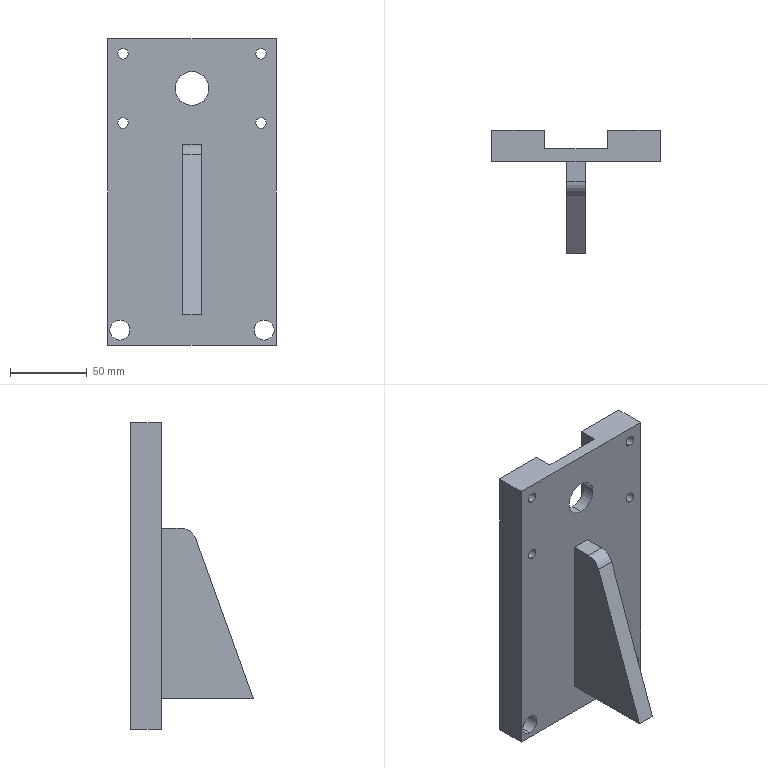Part | SolidWorks | features BaseBody 1 | 1 solid | 30 faces | box 110 x 80 x 200 mm | volume 383509 mm3 | cylinder 15 | plane 15 | commonest cylinder face diameters 6.8 x8 13 x4 22 x2 20 x1
STEP:
#1=CARTESIAN_POINT('',(178.,130.,-29.379));
#2=VERTEX_POINT('',#1);
#3=CARTESIAN_POINT('',(178.,130.,-16.379));
#4=VERTEX_POINT('',#3);
#5=CARTESIAN_POINT('',(178.,130.,-22.879));
#6=DIRECTION('',(0.,1.,0.));
#7=DIRECTION('',(0.,0.,1.));
#8=AXIS2_PLACEMENT_3D('',#5,#6,#7);
#9=CIRCLE('',#8,6.5);
#10=EDGE_CURVE('',#2,#4,#9,.T.);
#11=ORIENTED_EDGE('',*,*,#10,.F.);
#12=CARTESIAN_POINT('',(178.,150.,-29.379));
#13=VERTEX_POINT('',#12);
#14=CARTESIAN_POINT('',(178.,130.,-29.379));
#15=DIRECTION('',(0.,1.,0.));
#16=VECTOR('',#15,1000.);
#17=LINE('',#14,#16);
#18=EDGE_CURVE('',#2,#13,#17,.T.);
#19=ORIENTED_EDGE('',*,*,#18,.T.);
#20=CARTESIAN_POINT('',(178.,150.,-16.379));
#21=VERTEX_POINT('',#20);
#22=CARTESIAN_POINT('',(178.,150.,-22.879));
#23=DIRECTION('',(0.,-1.,0.));
#24=DIRECTION('',(0.,0.,1.));
#25=AXIS2_PLACEMENT_3D('',#22,#23,#24);
#26=CIRCLE('',#25,6.5);
#27=EDGE_CURVE('',#21,#13,#26,.T.);
#28=ORIENTED_EDGE('',*,*,#27,.F.);
#29=CARTESIAN_POINT('',(178.,130.,-16.379));
#30=DIRECTION('',(0.,1.,0.));
#31=VECTOR('',#30,1000.);
#32=LINE('',#29,#31);
#33=EDGE_CURVE('',#4,#21,#32,.T.);
#34=ORIENTED_EDGE('',*,*,#33,.F.);
#35=EDGE_LOOP('',(#11,#19,#28,#34));
#36=FACE_OUTER_BOUND('',#35,.T.);
#37=CARTESIAN_POINT('',(178.,130.,-22.879));
#38=DIRECTION('',(0.,1.,0.));
#39=DIRECTION('',(0.,0.,1.));
#40=AXIS2_PLACEMENT_3D('',#37,#38,#39);
#41=CYLINDRICAL_SURFACE('',#40,6.5);
#42=ADVANCED_FACE('',(#36),#41,.F.);
#43=CARTESIAN_POINT('',(272.,130.,-29.379));
#44=VERTEX_POINT('',#43);
#45=CARTESIAN_POINT('',(272.,130.,-16.379));
#46=VERTEX_POINT('',#45);
#47=CARTESIAN_POINT('',(272.,130.,-22.879));
#48=DIRECTION('',(0.,1.,0.));
#49=DIRECTION('',(0.,0.,1.));
#50=AXIS2_PLACEMENT_3D('',#47,#48,#49);
#51=CIRCLE('',#50,6.5);
#52=EDGE_CURVE('',#44,#46,#51,.T.);
#53=ORIENTED_EDGE('',*,*,#52,.F.);
#54=CARTESIAN_POINT('',(272.,150.,-29.379));
#55=VERTEX_POINT('',#54);
#56=CARTESIAN_POINT('',(272.,130.,-29.379));
#57=DIRECTION('',(0.,1.,0.));
#58=VECTOR('',#57,1000.);
#59=LINE('',#56,#58);
#60=EDGE_CURVE('',#44,#55,#59,.T.);
#61=ORIENTED_EDGE('',*,*,#60,.T.);
#62=CARTESIAN_POINT('',(272.,150.,-16.379));
#63=VERTEX_POINT('',#62);
#64=CARTESIAN_POINT('',(272.,150.,-22.879));
#65=DIRECTION('',(0.,-1.,0.));
#66=DIRECTION('',(0.,0.,1.));
#67=AXIS2_PLACEMENT_3D('',#64,#65,#66);
#68=CIRCLE('',#67,6.5);
#69=EDGE_CURVE('',#63,#55,#68,.T.);
#70=ORIENTED_EDGE('',*,*,#69,.F.);
#71=CARTESIAN_POINT('',(272.,130.,-16.379));
#72=DIRECTION('',(0.,1.,0.));
#73=VECTOR('',#72,1000.);
#74=LINE('',#71,#73);
#75=EDGE_CURVE('',#46,#63,#74,.T.);
#76=ORIENTED_EDGE('',*,*,#75,.F.);
#77=EDGE_LOOP('',(#53,#61,#70,#76));
#78=FACE_OUTER_BOUND('',#77,.T.);
#79=CARTESIAN_POINT('',(272.,130.,-22.879));
#80=DIRECTION('',(0.,1.,0.));
#81=DIRECTION('',(0.,0.,1.));
#82=AXIS2_PLACEMENT_3D('',#79,#80,#81);
#83=CYLINDRICAL_SURFACE('',#82,6.5);
#84=ADVANCED_FACE('',(#78),#83,.F.);
#85=CARTESIAN_POINT('',(270.,130.,108.721));
#86=VERTEX_POINT('',#85);
#87=CARTESIAN_POINT('',(270.,130.,115.521));
#88=VERTEX_POINT('',#87);
#89=CARTESIAN_POINT('',(270.,130.,112.121));
#90=DIRECTION('',(0.,1.,0.));
#91=DIRECTION('',(0.,0.,1.));
#92=AXIS2_PLACEMENT_3D('',#89,#90,#91);
#93=CIRCLE('',#92,3.4);
#94=EDGE_CURVE('',#86,#88,#93,.T.);
#95=ORIENTED_EDGE('',*,*,#94,.F.);
#96=CARTESIAN_POINT('',(270.,150.,108.721));
#97=VERTEX_POINT('',#96);
#98=CARTESIAN_POINT('',(270.,150.,108.721));
#99=DIRECTION('',(0.,1.,0.));
#100=VECTOR('',#99,1000.);
#101=LINE('',#98,#100);
#102=EDGE_CURVE('',#86,#97,#101,.T.);
#103=ORIENTED_EDGE('',*,*,#102,.T.);
#104=CARTESIAN_POINT('',(270.,150.,115.521));
#105=VERTEX_POINT('',#104);
#106=CARTESIAN_POINT('',(270.,150.,112.121));
#107=DIRECTION('',(0.,-1.,0.));
#108=DIRECTION('',(0.,0.,1.));
#109=AXIS2_PLACEMENT_3D('',#106,#107,#108);
#110=CIRCLE('',#109,3.4);
#111=EDGE_CURVE('',#105,#97,#110,.T.);
#112=ORIENTED_EDGE('',*,*,#111,.F.);
#113=CARTESIAN_POINT('',(270.,150.,115.521));
#114=DIRECTION('',(0.,1.,0.));
#115=VECTOR('',#114,1000.);
#116=LINE('',#113,#115);
#117=EDGE_CURVE('',#88,#105,#116,.T.);
#118=ORIENTED_EDGE('',*,*,#117,.F.);
#119=EDGE_LOOP('',(#95,#103,#112,#118));
#120=FACE_OUTER_BOUND('',#119,.T.);
#121=CARTESIAN_POINT('',(270.,150.,112.121));
#122=DIRECTION('',(0.,1.,0.));
#123=DIRECTION('',(0.,0.,1.));
#124=AXIS2_PLACEMENT_3D('',#121,#122,#123);
#125=CYLINDRICAL_SURFACE('',#124,3.4);
#126=ADVANCED_FACE('',(#120),#125,.F.);
#127=CARTESIAN_POINT('',(270.,130.,153.721));
#128=VERTEX_POINT('',#127);
#129=CARTESIAN_POINT('',(270.,130.,160.521));
#130=VERTEX_POINT('',#129);
#131=CARTESIAN_POINT('',(270.,130.,157.121));
#132=DIRECTION('',(0.,1.,0.));
#133=DIRECTION('',(0.,0.,1.));
#134=AXIS2_PLACEMENT_3D('',#131,#132,#133);
#135=CIRCLE('',#134,3.4);
#136=EDGE_CURVE('',#128,#130,#135,.T.);
#137=ORIENTED_EDGE('',*,*,#136,.F.);
#138=CARTESIAN_POINT('',(270.,150.,153.721));
#139=VERTEX_POINT('',#138);
#140=CARTESIAN_POINT('',(270.,150.,153.721));
#141=DIRECTION('',(0.,1.,0.));
#142=VECTOR('',#141,1000.);
#143=LINE('',#140,#142);
#144=EDGE_CURVE('',#128,#139,#143,.T.);
#145=ORIENTED_EDGE('',*,*,#144,.T.);
#146=CARTESIAN_POINT('',(270.,150.,160.521));
#147=VERTEX_POINT('',#146);
#148=CARTESIAN_POINT('',(270.,150.,157.121));
#149=DIRECTION('',(0.,-1.,0.));
#150=DIRECTION('',(0.,0.,1.));
#151=AXIS2_PLACEMENT_3D('',#148,#149,#150);
#152=CIRCLE('',#151,3.4);
#153=EDGE_CURVE('',#147,#139,#152,.T.);
#154=ORIENTED_EDGE('',*,*,#153,.F.);
#155=CARTESIAN_POINT('',(270.,150.,160.521));
#156=DIRECTION('',(0.,1.,0.));
#157=VECTOR('',#156,1000.);
#158=LINE('',#155,#157);
#159=EDGE_CURVE('',#130,#147,#158,.T.);
#160=ORIENTED_EDGE('',*,*,#159,.F.);
#161=EDGE_LOOP('',(#137,#145,#154,#160));
#162=FACE_OUTER_BOUND('',#161,.T.);
#163=CARTESIAN_POINT('',(270.,150.,157.121));
#164=DIRECTION('',(0.,1.,0.));
#165=DIRECTION('',(0.,0.,1.));
#166=AXIS2_PLACEMENT_3D('',#163,#164,#165);
#167=CYLINDRICAL_SURFACE('',#166,3.4);
#168=ADVANCED_FACE('',(#162),#167,.F.);
#169=CARTESIAN_POINT('',(180.,130.,108.721));
#170=VERTEX_POINT('',#169);
#171=CARTESIAN_POINT('',(180.,130.,115.521));
#172=VERTEX_POINT('',#171);
#173=CARTESIAN_POINT('',(180.,130.,112.121));
#174=DIRECTION('',(0.,1.,0.));
#175=DIRECTION('',(0.,0.,1.));
#176=AXIS2_PLACEMENT_3D('',#173,#174,#175);
#177=CIRCLE('',#176,3.4);
#178=EDGE_CURVE('',#170,#172,#177,.T.);
#179=ORIENTED_EDGE('',*,*,#178,.F.);
#180=CARTESIAN_POINT('',(180.,150.,108.721));
#181=VERTEX_POINT('',#180);
#182=CARTESIAN_POINT('',(180.,150.,108.721));
#183=DIRECTION('',(0.,1.,0.));
#184=VECTOR('',#183,1000.);
#185=LINE('',#182,#184);
#186=EDGE_CURVE('',#170,#181,#185,.T.);
#187=ORIENTED_EDGE('',*,*,#186,.T.);
#188=CARTESIAN_POINT('',(180.,150.,115.521));
#189=VERTEX_POINT('',#188);
#190=CARTESIAN_POINT('',(180.,150.,112.121));
#191=DIRECTION('',(0.,-1.,0.));
#192=DIRECTION('',(0.,0.,1.));
#193=AXIS2_PLACEMENT_3D('',#190,#191,#192);
#194=CIRCLE('',#193,3.4);
#195=EDGE_CURVE('',#189,#181,#194,.T.);
#196=ORIENTED_EDGE('',*,*,#195,.F.);
#197=CARTESIAN_POINT('',(180.,150.,115.521));
#198=DIRECTION('',(0.,1.,0.));
#199=VECTOR('',#198,1000.);
#200=LINE('',#197,#199);
#201=EDGE_CURVE('',#172,#189,#200,.T.);
#202=ORIENTED_EDGE('',*,*,#201,.F.);
#203=EDGE_LOOP('',(#179,#187,#196,#202));
#204=FACE_OUTER_BOUND('',#203,.T.);
#205=CARTESIAN_POINT('',(180.,150.,112.121));
#206=DIRECTION('',(0.,1.,0.));
#207=DIRECTION('',(0.,0.,1.));
#208=AXIS2_PLACEMENT_3D('',#205,#206,#207);
#209=CYLINDRICAL_SURFACE('',#208,3.4);
#210=ADVANCED_FACE('',(#204),#209,.F.);
#211=CARTESIAN_POINT('',(180.,130.,153.721));
#212=VERTEX_POINT('',#211);
#213=CARTESIAN_POINT('',(180.,130.,160.521));
#214=VERTEX_POINT('',#213);
#215=CARTESIAN_POINT('',(180.,130.,157.121));
#216=DIRECTION('',(0.,1.,0.));
#217=DIRECTION('',(0.,0.,1.));
#218=AXIS2_PLACEMENT_3D('',#215,#216,#217);
#219=CIRCLE('',#218,3.4);
#220=EDGE_CURVE('',#212,#214,#219,.T.);
#221=ORIENTED_EDGE('',*,*,#220,.F.);
#222=CARTESIAN_POINT('',(180.,150.,153.721));
#223=VERTEX_POINT('',#222);
#224=CARTESIAN_POINT('',(180.,150.,153.721));
#225=DIRECTION('',(0.,1.,0.));
#226=VECTOR('',#225,1000.);
#227=LINE('',#224,#226);
#228=EDGE_CURVE('',#212,#223,#227,.T.);
#229=ORIENTED_EDGE('',*,*,#228,.T.);
#230=CARTESIAN_POINT('',(180.,150.,160.521));
#231=VERTEX_POINT('',#230);
#232=CARTESIAN_POINT('',(180.,150.,157.121));
#233=DIRECTION('',(0.,-1.,0.));
#234=DIRECTION('',(0.,0.,1.));
#235=AXIS2_PLACEMENT_3D('',#232,#233,#234);
#236=CIRCLE('',#235,3.4);
#237=EDGE_CURVE('',#231,#223,#236,.T.);
#238=ORIENTED_EDGE('',*,*,#237,.F.);
#239=CARTESIAN_POINT('',(180.,150.,160.521));
#240=DIRECTION('',(0.,1.,0.));
#241=VECTOR('',#240,1000.);
#242=LINE('',#239,#241);
#243=EDGE_CURVE('',#214,#231,#242,.T.);
#244=ORIENTED_EDGE('',*,*,#243,.F.);
#245=EDGE_LOOP('',(#221,#229,#238,#244));
#246=FACE_OUTER_BOUND('',#245,.T.);
#247=CARTESIAN_POINT('',(180.,150.,157.121));
#248=DIRECTION('',(0.,1.,0.));
#249=DIRECTION('',(0.,0.,1.));
#250=AXIS2_PLACEMENT_3D('',#247,#248,#249);
#251=CYLINDRICAL_SURFACE('',#250,3.4);
#252=ADVANCED_FACE('',(#246),#251,.F.);
#253=CARTESIAN_POINT('',(225.,130.,123.621));
#254=VERTEX_POINT('',#253);
#255=CARTESIAN_POINT('',(225.,130.,145.621));
#256=VERTEX_POINT('',#255);
#257=CARTESIAN_POINT('',(225.,130.,134.621));
#258=DIRECTION('',(0.,1.,0.));
#259=DIRECTION('',(0.,0.,1.));
#260=AXIS2_PLACEMENT_3D('',#257,#258,#259);
#261=CIRCLE('',#260,11.);
#262=EDGE_CURVE('',#254,#256,#261,.T.);
#263=ORIENTED_EDGE('',*,*,#262,.F.);
#264=CARTESIAN_POINT('',(225.,138.,123.621));
#265=VERTEX_POINT('',#264);
#266=CARTESIAN_POINT('',(225.,129.999,123.621));
#267=DIRECTION('',(0.,1.,0.));
#268=VECTOR('',#267,1000.);
#269=LINE('',#266,#268);
#270=EDGE_CURVE('',#254,#265,#269,.T.);
#271=ORIENTED_EDGE('',*,*,#270,.T.);
#272=CARTESIAN_POINT('',(225.,138.,145.621));
#273=VERTEX_POINT('',#272);
#274=CARTESIAN_POINT('',(225.,138.,134.621));
#275=DIRECTION('',(0.,-1.,0.));
#276=DIRECTION('',(0.,0.,1.));
#277=AXIS2_PLACEMENT_3D('',#274,#275,#276);
#278=CIRCLE('',#277,11.);
#279=EDGE_CURVE('',#273,#265,#278,.T.);
#280=ORIENTED_EDGE('',*,*,#279,.F.);
#281=CARTESIAN_POINT('',(225.,129.999,145.621));
#282=DIRECTION('',(0.,1.,0.));
#283=VECTOR('',#282,1000.);
#284=LINE('',#281,#283);
#285=EDGE_CURVE('',#256,#273,#284,.T.);
#286=ORIENTED_EDGE('',*,*,#285,.F.);
#287=EDGE_LOOP('',(#263,#271,#280,#286));
#288=FACE_OUTER_BOUND('',#287,.T.);
#289=CARTESIAN_POINT('',(225.,129.999,134.621));
#290=DIRECTION('',(0.,1.,0.));
#291=DIRECTION('',(0.,0.,1.));
#292=AXIS2_PLACEMENT_3D('',#289,#290,#291);
#293=CYLINDRICAL_SURFACE('',#292,11.);
#294=ADVANCED_FACE('',(#288),#293,.F.);
#295=CARTESIAN_POINT('',(231.,130.,-12.879));
#296=VERTEX_POINT('',#295);
#297=CARTESIAN_POINT('',(219.,130.,-12.879));
#298=VERTEX_POINT('',#297);
#299=CARTESIAN_POINT('',(225.,130.,-12.879));
#300=DIRECTION('',(-1.,0.,0.));
#301=VECTOR('',#300,1000.);
#302=LINE('',#299,#301);
#303=EDGE_CURVE('',#296,#298,#302,.T.);
#304=ORIENTED_EDGE('',*,*,#303,.T.);
#305=CARTESIAN_POINT('',(219.,130.,98.107));
#306=VERTEX_POINT('',#305);
#307=CARTESIAN_POINT('',(219.,130.,67.121));
#308=DIRECTION('',(0.,0.,1.));
#309=VECTOR('',#308,1000.);
#310=LINE('',#307,#309);
#311=EDGE_CURVE('',#298,#306,#310,.T.);
#312=ORIENTED_EDGE('',*,*,#311,.T.);
#313=CARTESIAN_POINT('',(231.,130.,98.107));
#314=VERTEX_POINT('',#313);
#315=CARTESIAN_POINT('',(225.,130.,98.107));
#316=DIRECTION('',(1.,0.,0.));
#317=VECTOR('',#316,1000.);
#318=LINE('',#315,#317);
#319=EDGE_CURVE('',#306,#314,#318,.T.);
#320=ORIENTED_EDGE('',*,*,#319,.T.);
#321=CARTESIAN_POINT('',(231.,130.,67.121));
#322=DIRECTION('',(0.,0.,-1.));
#323=VECTOR('',#322,1000.);
#324=LINE('',#321,#323);
#325=EDGE_CURVE('',#314,#296,#324,.T.);
#326=ORIENTED_EDGE('',*,*,#325,.T.);
#327=EDGE_LOOP('',(#304,#312,#320,#326));
#328=FACE_BOUND('',#327,.T.);
#329=CARTESIAN_POINT('',(178.,130.,-22.879));
#330=DIRECTION('',(0.,1.,0.));
#331=DIRECTION('',(0.,0.,1.));
#332=AXIS2_PLACEMENT_3D('',#329,#330,#331);
#333=CIRCLE('',#332,6.5);
#334=EDGE_CURVE('',#4,#2,#333,.T.);
#335=ORIENTED_EDGE('',*,*,#334,.T.);
#336=ORIENTED_EDGE('',*,*,#10,.T.);
#337=EDGE_LOOP('',(#335,#336));
#338=FACE_BOUND('',#337,.T.);
#339=CARTESIAN_POINT('',(272.,130.,-22.879));
#340=DIRECTION('',(0.,1.,0.));
#341=DIRECTION('',(0.,0.,1.));
#342=AXIS2_PLACEMENT_3D('',#339,#340,#341);
#343=CIRCLE('',#342,6.5);
#344=EDGE_CURVE('',#46,#44,#343,.T.);
#345=ORIENTED_EDGE('',*,*,#344,.T.);
#346=ORIENTED_EDGE('',*,*,#52,.T.);
#347=EDGE_LOOP('',(#345,#346));
#348=FACE_BOUND('',#347,.T.);
#349=CARTESIAN_POINT('',(270.,130.,112.121));
#350=DIRECTION('',(0.,1.,0.));
#351=DIRECTION('',(0.,0.,1.));
#352=AXIS2_PLACEMENT_3D('',#349,#350,#351);
#353=CIRCLE('',#352,3.4);
#354=EDGE_CURVE('',#88,#86,#353,.T.);
#355=ORIENTED_EDGE('',*,*,#354,.T.);
#356=ORIENTED_EDGE('',*,*,#94,.T.);
#357=EDGE_LOOP('',(#355,#356));
#358=FACE_BOUND('',#357,.T.);
#359=CARTESIAN_POINT('',(270.,130.,157.121));
#360=DIRECTION('',(0.,1.,0.));
#361=DIRECTION('',(0.,0.,1.));
#362=AXIS2_PLACEMENT_3D('',#359,#360,#361);
#363=CIRCLE('',#362,3.4);
#364=EDGE_CURVE('',#130,#128,#363,.T.);
#365=ORIENTED_EDGE('',*,*,#364,.T.);
#366=ORIENTED_EDGE('',*,*,#136,.T.);
#367=EDGE_LOOP('',(#365,#366));
#368=FACE_BOUND('',#367,.T.);
#369=CARTESIAN_POINT('',(180.,130.,112.121));
#370=DIRECTION('',(0.,1.,0.));
#371=DIRECTION('',(0.,0.,1.));
#372=AXIS2_PLACEMENT_3D('',#369,#370,#371);
#373=CIRCLE('',#372,3.4);
#374=EDGE_CURVE('',#172,#170,#373,.T.);
#375=ORIENTED_EDGE('',*,*,#374,.T.);
#376=ORIENTED_EDGE('',*,*,#178,.T.);
#377=EDGE_LOOP('',(#375,#376));
#378=FACE_BOUND('',#377,.T.);
#379=CARTESIAN_POINT('',(180.,130.,157.121));
#380=DIRECTION('',(0.,1.,0.));
#381=DIRECTION('',(0.,0.,1.));
#382=AXIS2_PLACEMENT_3D('',#379,#380,#381);
#383=CIRCLE('',#382,3.4);
#384=EDGE_CURVE('',#214,#212,#383,.T.);
#385=ORIENTED_EDGE('',*,*,#384,.T.);
#386=ORIENTED_EDGE('',*,*,#220,.T.);
#387=EDGE_LOOP('',(#385,#386));
#388=FACE_BOUND('',#387,.T.);
#389=CARTESIAN_POINT('',(225.,130.,134.621));
#390=DIRECTION('',(0.,1.,0.));
#391=DIRECTION('',(0.,0.,1.));
#392=AXIS2_PLACEMENT_3D('',#389,#390,#391);
#393=CIRCLE('',#392,11.);
#394=EDGE_CURVE('',#256,#254,#393,.T.);
#395=ORIENTED_EDGE('',*,*,#394,.T.);
#396=ORIENTED_EDGE('',*,*,#262,.T.);
#397=EDGE_LOOP('',(#395,#396));
#398=FACE_BOUND('',#397,.T.);
#399=CARTESIAN_POINT('',(170.,130.,167.121));
#400=VERTEX_POINT('',#399);
#401=CARTESIAN_POINT('',(170.,130.,-32.879));
#402=VERTEX_POINT('',#401);
#403=CARTESIAN_POINT('',(170.,130.,67.121));
#404=DIRECTION('',(0.,0.,-1.));
#405=VECTOR('',#404,1000.);
#406=LINE('',#403,#405);
#407=EDGE_CURVE('',#400,#402,#406,.T.);
#408=ORIENTED_EDGE('',*,*,#407,.T.);
#409=CARTESIAN_POINT('',(280.,130.,-32.879));
#410=VERTEX_POINT('',#409);
#411=CARTESIAN_POINT('',(225.,130.,-32.879));
#412=DIRECTION('',(1.,0.,0.));
#413=VECTOR('',#412,1000.);
#414=LINE('',#411,#413);
#415=EDGE_CURVE('',#402,#410,#414,.T.);
#416=ORIENTED_EDGE('',*,*,#415,.T.);
#417=CARTESIAN_POINT('',(280.,130.,167.121));
#418=VERTEX_POINT('',#417);
#419=CARTESIAN_POINT('',(280.,130.,67.121));
#420=DIRECTION('',(0.,0.,1.));
#421=VECTOR('',#420,1000.);
#422=LINE('',#419,#421);
#423=EDGE_CURVE('',#410,#418,#422,.T.);
#424=ORIENTED_EDGE('',*,*,#423,.T.);
#425=CARTESIAN_POINT('',(225.,130.,167.121));
#426=DIRECTION('',(-1.,0.,0.));
#427=VECTOR('',#426,1000.);
#428=LINE('',#425,#427);
#429=EDGE_CURVE('',#418,#400,#428,.T.);
#430=ORIENTED_EDGE('',*,*,#429,.T.);
#431=EDGE_LOOP('',(#408,#416,#424,#430));
#432=FACE_OUTER_BOUND('',#431,.T.);
#433=CARTESIAN_POINT('',(225.,130.,67.121));
#434=DIRECTION('',(0.,-1.,0.));
#435=DIRECTION('',(0.,0.,-1.));
#436=AXIS2_PLACEMENT_3D('',#433,#434,#435);
#437=PLANE('',#436);
#438=ADVANCED_FACE('',(#328,#338,#348,#358,#368,#378,#388,#398,#432),#437,.T.);
#439=ORIENTED_EDGE('',*,*,#311,.F.);
#440=CARTESIAN_POINT('',(219.,70.,-12.879));
#441=VERTEX_POINT('',#440);
#442=CARTESIAN_POINT('',(219.,130.,-12.879));
#443=DIRECTION('',(0.,-1.,0.));
#444=VECTOR('',#443,1000.);
#445=LINE('',#442,#444);
#446=EDGE_CURVE('',#298,#441,#445,.T.);
#447=ORIENTED_EDGE('',*,*,#446,.T.);
#448=CARTESIAN_POINT('',(219.,107.618,91.497));
#449=VERTEX_POINT('',#448);
#450=CARTESIAN_POINT('',(219.,70.,-12.879));
#451=DIRECTION('',(0.,0.3391,0.9408));
#452=VECTOR('',#451,1000.);
#453=LINE('',#450,#452);
#454=EDGE_CURVE('',#441,#449,#453,.T.);
#455=ORIENTED_EDGE('',*,*,#454,.T.);
#456=CARTESIAN_POINT('',(219.,117.026,98.107));
#457=VERTEX_POINT('',#456);
#458=CARTESIAN_POINT('',(219.,117.026,88.107));
#459=DIRECTION('',(-1.,0.,0.));
#460=DIRECTION('',(0.,0.,1.));
#461=AXIS2_PLACEMENT_3D('',#458,#459,#460);
#462=CIRCLE('',#461,10.);
#463=EDGE_CURVE('',#449,#457,#462,.T.);
#464=ORIENTED_EDGE('',*,*,#463,.T.);
#465=CARTESIAN_POINT('',(219.,130.,98.107));
#466=DIRECTION('',(0.,1.,0.));
#467=VECTOR('',#466,1000.);
#468=LINE('',#465,#467);
#469=EDGE_CURVE('',#457,#306,#468,.T.);
#470=ORIENTED_EDGE('',*,*,#469,.T.);
#471=EDGE_LOOP('',(#439,#447,#455,#464,#470));
#472=FACE_OUTER_BOUND('',#471,.T.);
#473=CARTESIAN_POINT('',(219.,130.,67.121));
#474=DIRECTION('',(-1.,0.,0.));
#475=DIRECTION('',(0.,0.,1.));
#476=AXIS2_PLACEMENT_3D('',#473,#474,#475);
#477=PLANE('',#476);
#478=ADVANCED_FACE('',(#472),#477,.T.);
#479=ORIENTED_EDGE('',*,*,#303,.F.);
#480=CARTESIAN_POINT('',(231.,70.,-12.879));
#481=VERTEX_POINT('',#480);
#482=CARTESIAN_POINT('',(231.,130.,-12.879));
#483=DIRECTION('',(0.,1.,0.));
#484=VECTOR('',#483,1000.);
#485=LINE('',#482,#484);
#486=EDGE_CURVE('',#481,#296,#485,.T.);
#487=ORIENTED_EDGE('',*,*,#486,.F.);
#488=CARTESIAN_POINT('',(231.,70.,-12.879));
#489=DIRECTION('',(1.,0.,0.));
#490=VECTOR('',#489,1000.);
#491=LINE('',#488,#490);
#492=EDGE_CURVE('',#441,#481,#491,.T.);
#493=ORIENTED_EDGE('',*,*,#492,.F.);
#494=ORIENTED_EDGE('',*,*,#446,.F.);
#495=EDGE_LOOP('',(#479,#487,#493,#494));
#496=FACE_OUTER_BOUND('',#495,.T.);
#497=CARTESIAN_POINT('',(231.,130.,-12.879));
#498=DIRECTION('',(0.,0.,1.));
#499=DIRECTION('',(1.,0.,0.));
#500=AXIS2_PLACEMENT_3D('',#497,#498,#499);
#501=PLANE('',#500);
#502=ADVANCED_FACE('',(#496),#501,.F.);
#503=CARTESIAN_POINT('',(231.,107.618,91.497));
#504=VERTEX_POINT('',#503);
#505=CARTESIAN_POINT('',(231.,117.026,98.107));
#506=VERTEX_POINT('',#505);
#507=CARTESIAN_POINT('',(231.,117.026,88.107));
#508=DIRECTION('',(-1.,0.,0.));
#509=DIRECTION('',(0.,0.,1.));
#510=AXIS2_PLACEMENT_3D('',#507,#508,#509);
#511=CIRCLE('',#510,10.);
#512=EDGE_CURVE('',#504,#506,#511,.T.);
#513=ORIENTED_EDGE('',*,*,#512,.F.);
#514=CARTESIAN_POINT('',(231.,70.,-12.879));
#515=DIRECTION('',(0.,0.3391,0.9408));
#516=VECTOR('',#515,1000.);
#517=LINE('',#514,#516);
#518=EDGE_CURVE('',#481,#504,#517,.T.);
#519=ORIENTED_EDGE('',*,*,#518,.F.);
#520=ORIENTED_EDGE('',*,*,#486,.T.);
#521=ORIENTED_EDGE('',*,*,#325,.F.);
#522=CARTESIAN_POINT('',(231.,130.,98.107));
#523=DIRECTION('',(0.,1.,0.));
#524=VECTOR('',#523,1000.);
#525=LINE('',#522,#524);
#526=EDGE_CURVE('',#506,#314,#525,.T.);
#527=ORIENTED_EDGE('',*,*,#526,.F.);
#528=EDGE_LOOP('',(#513,#519,#520,#521,#527));
#529=FACE_OUTER_BOUND('',#528,.T.);
#530=CARTESIAN_POINT('',(231.,130.,67.121));
#531=DIRECTION('',(-1.,0.,0.));
#532=DIRECTION('',(0.,0.,1.));
#533=AXIS2_PLACEMENT_3D('',#530,#531,#532);
#534=PLANE('',#533);
#535=ADVANCED_FACE('',(#529),#534,.F.);
#536=CARTESIAN_POINT('',(231.,117.026,98.107));
#537=DIRECTION('',(-1.,0.,0.));
#538=VECTOR('',#537,1000.);
#539=LINE('',#536,#538);
#540=EDGE_CURVE('',#506,#457,#539,.T.);
#541=ORIENTED_EDGE('',*,*,#540,.F.);
#542=ORIENTED_EDGE('',*,*,#526,.T.);
#543=ORIENTED_EDGE('',*,*,#319,.F.);
#544=ORIENTED_EDGE('',*,*,#469,.F.);
#545=EDGE_LOOP('',(#541,#542,#543,#544));
#546=FACE_OUTER_BOUND('',#545,.T.);
#547=CARTESIAN_POINT('',(231.,130.,98.107));
#548=DIRECTION('',(0.,0.,-1.));
#549=DIRECTION('',(-1.,0.,0.));
#550=AXIS2_PLACEMENT_3D('',#547,#548,#549);
#551=PLANE('',#550);
#552=ADVANCED_FACE('',(#546),#551,.F.);
#553=ORIENTED_EDGE('',*,*,#18,.F.);
#554=ORIENTED_EDGE('',*,*,#334,.F.);
#555=ORIENTED_EDGE('',*,*,#33,.T.);
#556=CARTESIAN_POINT('',(178.,150.,-22.879));
#557=DIRECTION('',(0.,-1.,0.));
#558=DIRECTION('',(0.,0.,1.));
#559=AXIS2_PLACEMENT_3D('',#556,#557,#558);
#560=CIRCLE('',#559,6.5);
#561=EDGE_CURVE('',#13,#21,#560,.T.);
#562=ORIENTED_EDGE('',*,*,#561,.F.);
#563=EDGE_LOOP('',(#553,#554,#555,#562));
#564=FACE_OUTER_BOUND('',#563,.T.);
#565=CARTESIAN_POINT('',(178.,130.,-22.879));
#566=DIRECTION('',(0.,1.,0.));
#567=DIRECTION('',(0.,0.,1.));
#568=AXIS2_PLACEMENT_3D('',#565,#566,#567);
#569=CYLINDRICAL_SURFACE('',#568,6.5);
#570=ADVANCED_FACE('',(#564),#569,.F.);
#571=ORIENTED_EDGE('',*,*,#60,.F.);
#572=ORIENTED_EDGE('',*,*,#344,.F.);
#573=ORIENTED_EDGE('',*,*,#75,.T.);
#574=CARTESIAN_POINT('',(272.,150.,-22.879));
#575=DIRECTION('',(0.,-1.,0.));
#576=DIRECTION('',(0.,0.,1.));
#577=AXIS2_PLACEMENT_3D('',#574,#575,#576);
#578=CIRCLE('',#577,6.5);
#579=EDGE_CURVE('',#55,#63,#578,.T.);
#580=ORIENTED_EDGE('',*,*,#579,.F.);
#581=EDGE_LOOP('',(#571,#572,#573,#580));
#582=FACE_OUTER_BOUND('',#581,.T.);
#583=CARTESIAN_POINT('',(272.,130.,-22.879));
#584=DIRECTION('',(0.,1.,0.));
#585=DIRECTION('',(0.,0.,1.));
#586=AXIS2_PLACEMENT_3D('',#583,#584,#585);
#587=CYLINDRICAL_SURFACE('',#586,6.5);
#588=ADVANCED_FACE('',(#582),#587,.F.);
#589=ORIENTED_EDGE('',*,*,#102,.F.);
#590=ORIENTED_EDGE('',*,*,#354,.F.);
#591=ORIENTED_EDGE('',*,*,#117,.T.);
#592=CARTESIAN_POINT('',(270.,150.,112.121));
#593=DIRECTION('',(0.,-1.,0.));
#594=DIRECTION('',(0.,0.,1.));
#595=AXIS2_PLACEMENT_3D('',#592,#593,#594);
#596=CIRCLE('',#595,3.4);
#597=EDGE_CURVE('',#97,#105,#596,.T.);
#598=ORIENTED_EDGE('',*,*,#597,.F.);
#599=EDGE_LOOP('',(#589,#590,#591,#598));
#600=FACE_OUTER_BOUND('',#599,.T.);
#601=CARTESIAN_POINT('',(270.,150.,112.121));
#602=DIRECTION('',(0.,1.,0.));
#603=DIRECTION('',(0.,0.,1.));
#604=AXIS2_PLACEMENT_3D('',#601,#602,#603);
#605=CYLINDRICAL_SURFACE('',#604,3.4);
#606=ADVANCED_FACE('',(#600),#605,.F.);
#607=ORIENTED_EDGE('',*,*,#144,.F.);
#608=ORIENTED_EDGE('',*,*,#364,.F.);
#609=ORIENTED_EDGE('',*,*,#159,.T.);
#610=CARTESIAN_POINT('',(270.,150.,157.121));
#611=DIRECTION('',(0.,-1.,0.));
#612=DIRECTION('',(0.,0.,1.));
#613=AXIS2_PLACEMENT_3D('',#610,#611,#612);
#614=CIRCLE('',#613,3.4);
#615=EDGE_CURVE('',#139,#147,#614,.T.);
#616=ORIENTED_EDGE('',*,*,#615,.F.);
#617=EDGE_LOOP('',(#607,#608,#609,#616));
#618=FACE_OUTER_BOUND('',#617,.T.);
#619=CARTESIAN_POINT('',(270.,150.,157.121));
#620=DIRECTION('',(0.,1.,0.));
#621=DIRECTION('',(0.,0.,1.));
#622=AXIS2_PLACEMENT_3D('',#619,#620,#621);
#623=CYLINDRICAL_SURFACE('',#622,3.4);
#624=ADVANCED_FACE('',(#618),#623,.F.);
#625=ORIENTED_EDGE('',*,*,#186,.F.);
#626=ORIENTED_EDGE('',*,*,#374,.F.);
#627=ORIENTED_EDGE('',*,*,#201,.T.);
#628=CARTESIAN_POINT('',(180.,150.,112.121));
#629=DIRECTION('',(0.,-1.,0.));
#630=DIRECTION('',(0.,0.,1.));
#631=AXIS2_PLACEMENT_3D('',#628,#629,#630);
#632=CIRCLE('',#631,3.4);
#633=EDGE_CURVE('',#181,#189,#632,.T.);
#634=ORIENTED_EDGE('',*,*,#633,.F.);
#635=EDGE_LOOP('',(#625,#626,#627,#634));
#636=FACE_OUTER_BOUND('',#635,.T.);
#637=CARTESIAN_POINT('',(180.,150.,112.121));
#638=DIRECTION('',(0.,1.,0.));
#639=DIRECTION('',(0.,0.,1.));
#640=AXIS2_PLACEMENT_3D('',#637,#638,#639);
#641=CYLINDRICAL_SURFACE('',#640,3.4);
#642=ADVANCED_FACE('',(#636),#641,.F.);
#643=ORIENTED_EDGE('',*,*,#228,.F.);
#644=ORIENTED_EDGE('',*,*,#384,.F.);
#645=ORIENTED_EDGE('',*,*,#243,.T.);
#646=CARTESIAN_POINT('',(180.,150.,157.121));
#647=DIRECTION('',(0.,-1.,0.));
#648=DIRECTION('',(0.,0.,1.));
#649=AXIS2_PLACEMENT_3D('',#646,#647,#648);
#650=CIRCLE('',#649,3.4);
#651=EDGE_CURVE('',#223,#231,#650,.T.);
#652=ORIENTED_EDGE('',*,*,#651,.F.);
#653=EDGE_LOOP('',(#643,#644,#645,#652));
#654=FACE_OUTER_BOUND('',#653,.T.);
#655=CARTESIAN_POINT('',(180.,150.,157.121));
#656=DIRECTION('',(0.,1.,0.));
#657=DIRECTION('',(0.,0.,1.));
#658=AXIS2_PLACEMENT_3D('',#655,#656,#657);
#659=CYLINDRICAL_SURFACE('',#658,3.4);
#660=ADVANCED_FACE('',(#654),#659,.F.);
#661=ORIENTED_EDGE('',*,*,#270,.F.);
#662=ORIENTED_EDGE('',*,*,#394,.F.);
#663=ORIENTED_EDGE('',*,*,#285,.T.);
#664=CARTESIAN_POINT('',(225.,138.,134.621));
#665=DIRECTION('',(0.,-1.,0.));
#666=DIRECTION('',(0.,0.,1.));
#667=AXIS2_PLACEMENT_3D('',#664,#665,#666);
#668=CIRCLE('',#667,11.);
#669=EDGE_CURVE('',#265,#273,#668,.T.);
#670=ORIENTED_EDGE('',*,*,#669,.F.);
#671=EDGE_LOOP('',(#661,#662,#663,#670));
#672=FACE_OUTER_BOUND('',#671,.T.);
#673=CARTESIAN_POINT('',(225.,129.999,134.621));
#674=DIRECTION('',(0.,1.,0.));
#675=DIRECTION('',(0.,0.,1.));
#676=AXIS2_PLACEMENT_3D('',#673,#674,#675);
#677=CYLINDRICAL_SURFACE('',#676,11.);
#678=ADVANCED_FACE('',(#672),#677,.F.);
#679=CARTESIAN_POINT('',(245.5,150.,-32.879));
#680=VERTEX_POINT('',#679);
#681=CARTESIAN_POINT('',(245.5,138.,-32.879));
#682=VERTEX_POINT('',#681);
#683=CARTESIAN_POINT('',(245.5,150.,-32.879));
#684=DIRECTION('',(0.,-1.,0.));
#685=VECTOR('',#684,1000.);
#686=LINE('',#683,#685);
#687=EDGE_CURVE('',#680,#682,#686,.T.);
#688=ORIENTED_EDGE('',*,*,#687,.F.);
#689=CARTESIAN_POINT('',(280.,150.,-32.879));
#690=VERTEX_POINT('',#689);
#691=CARTESIAN_POINT('',(170.,150.,-32.879));
#692=DIRECTION('',(-1.,0.,0.));
#693=VECTOR('',#692,1000.);
#694=LINE('',#691,#693);
#695=EDGE_CURVE('',#690,#680,#694,.T.);
#696=ORIENTED_EDGE('',*,*,#695,.F.);
#697=CARTESIAN_POINT('',(280.,150.,-32.879));
#698=DIRECTION('',(0.,1.,0.));
#699=VECTOR('',#698,1000.);
#700=LINE('',#697,#699);
#701=EDGE_CURVE('',#410,#690,#700,.T.);
#702=ORIENTED_EDGE('',*,*,#701,.F.);
#703=ORIENTED_EDGE('',*,*,#415,.F.);
#704=CARTESIAN_POINT('',(170.,150.,-32.879));
#705=VERTEX_POINT('',#704);
#706=CARTESIAN_POINT('',(170.,150.,-32.879));
#707=DIRECTION('',(0.,-1.,0.));
#708=VECTOR('',#707,1000.);
#709=LINE('',#706,#708);
#710=EDGE_CURVE('',#705,#402,#709,.T.);
#711=ORIENTED_EDGE('',*,*,#710,.F.);
#712=CARTESIAN_POINT('',(204.5,150.,-32.879));
#713=VERTEX_POINT('',#712);
#714=CARTESIAN_POINT('',(170.,150.,-32.879));
#715=DIRECTION('',(-1.,0.,0.));
#716=VECTOR('',#715,1000.);
#717=LINE('',#714,#716);
#718=EDGE_CURVE('',#713,#705,#717,.T.);
#719=ORIENTED_EDGE('',*,*,#718,.F.);
#720=CARTESIAN_POINT('',(204.5,138.,-32.879));
#721=VERTEX_POINT('',#720);
#722=CARTESIAN_POINT('',(204.5,150.,-32.879));
#723=DIRECTION('',(0.,1.,0.));
#724=VECTOR('',#723,1000.);
#725=LINE('',#722,#724);
#726=EDGE_CURVE('',#721,#713,#725,.T.);
#727=ORIENTED_EDGE('',*,*,#726,.F.);
#728=CARTESIAN_POINT('',(170.,138.,-32.879));
#729=DIRECTION('',(-1.,0.,0.));
#730=VECTOR('',#729,1000.);
#731=LINE('',#728,#730);
#732=EDGE_CURVE('',#682,#721,#731,.T.);
#733=ORIENTED_EDGE('',*,*,#732,.F.);
#734=EDGE_LOOP('',(#688,#696,#702,#703,#711,#719,#727,#733));
#735=FACE_OUTER_BOUND('',#734,.T.);
#736=CARTESIAN_POINT('',(170.,150.,-32.879));
#737=DIRECTION('',(0.,0.,1.));
#738=DIRECTION('',(1.,0.,0.));
#739=AXIS2_PLACEMENT_3D('',#736,#737,#738);
#740=PLANE('',#739);
#741=ADVANCED_FACE('',(#735),#740,.F.);
#742=CARTESIAN_POINT('',(170.,150.,167.121));
#743=VERTEX_POINT('',#742);
#744=CARTESIAN_POINT('',(170.,150.,167.121));
#745=DIRECTION('',(0.,-1.,0.));
#746=VECTOR('',#745,1000.);
#747=LINE('',#744,#746);
#748=EDGE_CURVE('',#743,#400,#747,.T.);
#749=ORIENTED_EDGE('',*,*,#748,.F.);
#750=CARTESIAN_POINT('',(170.,150.,167.121));
#751=DIRECTION('',(0.,0.,1.));
#752=VECTOR('',#751,1000.);
#753=LINE('',#750,#752);
#754=EDGE_CURVE('',#705,#743,#753,.T.);
#755=ORIENTED_EDGE('',*,*,#754,.F.);
#756=ORIENTED_EDGE('',*,*,#710,.T.);
#757=ORIENTED_EDGE('',*,*,#407,.F.);
#758=EDGE_LOOP('',(#749,#755,#756,#757));
#759=FACE_OUTER_BOUND('',#758,.T.);
#760=CARTESIAN_POINT('',(170.,150.,167.121));
#761=DIRECTION('',(1.,0.,0.));
#762=DIRECTION('',(0.,0.,-1.));
#763=AXIS2_PLACEMENT_3D('',#760,#761,#762);
#764=PLANE('',#763);
#765=ADVANCED_FACE('',(#759),#764,.F.);
#766=CARTESIAN_POINT('',(245.5,138.,167.121));
#767=VERTEX_POINT('',#766);
#768=CARTESIAN_POINT('',(245.5,150.,167.121));
#769=VERTEX_POINT('',#768);
#770=CARTESIAN_POINT('',(245.5,150.,167.121));
#771=DIRECTION('',(0.,1.,0.));
#772=VECTOR('',#771,1000.);
#773=LINE('',#770,#772);
#774=EDGE_CURVE('',#767,#769,#773,.T.);
#775=ORIENTED_EDGE('',*,*,#774,.F.);
#776=CARTESIAN_POINT('',(204.5,138.,167.121));
#777=VERTEX_POINT('',#776);
#778=CARTESIAN_POINT('',(170.,138.,167.121));
#779=DIRECTION('',(1.,0.,0.));
#780=VECTOR('',#779,1000.);
#781=LINE('',#778,#780);
#782=EDGE_CURVE('',#777,#767,#781,.T.);
#783=ORIENTED_EDGE('',*,*,#782,.F.);
#784=CARTESIAN_POINT('',(204.5,150.,167.121));
#785=VERTEX_POINT('',#784);
#786=CARTESIAN_POINT('',(204.5,150.,167.121));
#787=DIRECTION('',(0.,-1.,0.));
#788=VECTOR('',#787,1000.);
#789=LINE('',#786,#788);
#790=EDGE_CURVE('',#785,#777,#789,.T.);
#791=ORIENTED_EDGE('',*,*,#790,.F.);
#792=CARTESIAN_POINT('',(170.,150.,167.121));
#793=DIRECTION('',(1.,0.,0.));
#794=VECTOR('',#793,1000.);
#795=LINE('',#792,#794);
#796=EDGE_CURVE('',#743,#785,#795,.T.);
#797=ORIENTED_EDGE('',*,*,#796,.F.);
#798=ORIENTED_EDGE('',*,*,#748,.T.);
#799=ORIENTED_EDGE('',*,*,#429,.F.);
#800=CARTESIAN_POINT('',(280.,150.,167.121));
#801=VERTEX_POINT('',#800);
#802=CARTESIAN_POINT('',(280.,150.,167.121));
#803=DIRECTION('',(0.,-1.,0.));
#804=VECTOR('',#803,1000.);
#805=LINE('',#802,#804);
#806=EDGE_CURVE('',#801,#418,#805,.T.);
#807=ORIENTED_EDGE('',*,*,#806,.F.);
#808=CARTESIAN_POINT('',(170.,150.,167.121));
#809=DIRECTION('',(1.,0.,0.));
#810=VECTOR('',#809,1000.);
#811=LINE('',#808,#810);
#812=EDGE_CURVE('',#769,#801,#811,.T.);
#813=ORIENTED_EDGE('',*,*,#812,.F.);
#814=EDGE_LOOP('',(#775,#783,#791,#797,#798,#799,#807,#813));
#815=FACE_OUTER_BOUND('',#814,.T.);
#816=CARTESIAN_POINT('',(170.,150.,167.121));
#817=DIRECTION('',(0.,0.,-1.));
#818=DIRECTION('',(-1.,0.,0.));
#819=AXIS2_PLACEMENT_3D('',#816,#817,#818);
#820=PLANE('',#819);
#821=ADVANCED_FACE('',(#815),#820,.F.);
#822=ORIENTED_EDGE('',*,*,#701,.T.);
#823=CARTESIAN_POINT('',(280.,150.,167.121));
#824=DIRECTION('',(0.,0.,-1.));
#825=VECTOR('',#824,1000.);
#826=LINE('',#823,#825);
#827=EDGE_CURVE('',#801,#690,#826,.T.);
#828=ORIENTED_EDGE('',*,*,#827,.F.);
#829=ORIENTED_EDGE('',*,*,#806,.T.);
#830=ORIENTED_EDGE('',*,*,#423,.F.);
#831=EDGE_LOOP('',(#822,#828,#829,#830));
#832=FACE_OUTER_BOUND('',#831,.T.);
#833=CARTESIAN_POINT('',(280.,150.,167.121));
#834=DIRECTION('',(-1.,0.,0.));
#835=DIRECTION('',(0.,0.,1.));
#836=AXIS2_PLACEMENT_3D('',#833,#834,#835);
#837=PLANE('',#836);
#838=ADVANCED_FACE('',(#832),#837,.F.);
#839=ORIENTED_EDGE('',*,*,#463,.F.);
#840=CARTESIAN_POINT('',(231.,107.618,91.497));
#841=DIRECTION('',(1.,0.,0.));
#842=VECTOR('',#841,1000.);
#843=LINE('',#840,#842);
#844=EDGE_CURVE('',#449,#504,#843,.T.);
#845=ORIENTED_EDGE('',*,*,#844,.T.);
#846=ORIENTED_EDGE('',*,*,#512,.T.);
#847=ORIENTED_EDGE('',*,*,#540,.T.);
#848=EDGE_LOOP('',(#839,#845,#846,#847));
#849=FACE_OUTER_BOUND('',#848,.T.);
#850=CARTESIAN_POINT('',(231.,117.026,88.107));
#851=DIRECTION('',(-1.,0.,0.));
#852=DIRECTION('',(0.,0.,1.));
#853=AXIS2_PLACEMENT_3D('',#850,#851,#852);
#854=CYLINDRICAL_SURFACE('',#853,10.);
#855=ADVANCED_FACE('',(#849),#854,.T.);
#856=ORIENTED_EDGE('',*,*,#844,.F.);
#857=ORIENTED_EDGE('',*,*,#454,.F.);
#858=ORIENTED_EDGE('',*,*,#492,.T.);
#859=ORIENTED_EDGE('',*,*,#518,.T.);
#860=EDGE_LOOP('',(#856,#857,#858,#859));
#861=FACE_OUTER_BOUND('',#860,.T.);
#862=CARTESIAN_POINT('',(231.,110.,98.107));
#863=DIRECTION('',(0.,0.9408,-0.3391));
#864=DIRECTION('',(0.,0.3391,0.9408));
#865=AXIS2_PLACEMENT_3D('',#862,#863,#864);
#866=PLANE('',#865);
#867=ADVANCED_FACE('',(#861),#866,.F.);
#868=CARTESIAN_POINT('',(204.5,150.,67.121));
#869=DIRECTION('',(0.,0.,1.));
#870=VECTOR('',#869,1000.);
#871=LINE('',#868,#870);
#872=EDGE_CURVE('',#713,#785,#871,.T.);
#873=ORIENTED_EDGE('',*,*,#872,.F.);
#874=ORIENTED_EDGE('',*,*,#718,.T.);
#875=ORIENTED_EDGE('',*,*,#754,.T.);
#876=ORIENTED_EDGE('',*,*,#796,.T.);
#877=EDGE_LOOP('',(#873,#874,#875,#876));
#878=FACE_OUTER_BOUND('',#877,.T.);
#879=ORIENTED_EDGE('',*,*,#237,.T.);
#880=ORIENTED_EDGE('',*,*,#651,.T.);
#881=EDGE_LOOP('',(#879,#880));
#882=FACE_BOUND('',#881,.T.);
#883=ORIENTED_EDGE('',*,*,#195,.T.);
#884=ORIENTED_EDGE('',*,*,#633,.T.);
#885=EDGE_LOOP('',(#883,#884));
#886=FACE_BOUND('',#885,.T.);
#887=ORIENTED_EDGE('',*,*,#27,.T.);
#888=ORIENTED_EDGE('',*,*,#561,.T.);
#889=EDGE_LOOP('',(#887,#888));
#890=FACE_BOUND('',#889,.T.);
#891=CARTESIAN_POINT('',(225.,150.,67.121));
#892=DIRECTION('',(0.,-1.,0.));
#893=DIRECTION('',(0.,0.,-1.));
#894=AXIS2_PLACEMENT_3D('',#891,#892,#893);
#895=PLANE('',#894);
#896=ADVANCED_FACE('',(#878,#882,#886,#890),#895,.F.);
#897=CARTESIAN_POINT('',(245.5,150.,67.121));
#898=DIRECTION('',(0.,0.,-1.));
#899=VECTOR('',#898,1000.);
#900=LINE('',#897,#899);
#901=EDGE_CURVE('',#769,#680,#900,.T.);
#902=ORIENTED_EDGE('',*,*,#901,.F.);
#903=ORIENTED_EDGE('',*,*,#812,.T.);
#904=ORIENTED_EDGE('',*,*,#827,.T.);
#905=ORIENTED_EDGE('',*,*,#695,.T.);
#906=EDGE_LOOP('',(#902,#903,#904,#905));
#907=FACE_OUTER_BOUND('',#906,.T.);
#908=ORIENTED_EDGE('',*,*,#153,.T.);
#909=ORIENTED_EDGE('',*,*,#615,.T.);
#910=EDGE_LOOP('',(#908,#909));
#911=FACE_BOUND('',#910,.T.);
#912=ORIENTED_EDGE('',*,*,#111,.T.);
#913=ORIENTED_EDGE('',*,*,#597,.T.);
#914=EDGE_LOOP('',(#912,#913));
#915=FACE_BOUND('',#914,.T.);
#916=ORIENTED_EDGE('',*,*,#69,.T.);
#917=ORIENTED_EDGE('',*,*,#579,.T.);
#918=EDGE_LOOP('',(#916,#917));
#919=FACE_BOUND('',#918,.T.);
#920=CARTESIAN_POINT('',(225.,150.,67.121));
#921=DIRECTION('',(0.,-1.,0.));
#922=DIRECTION('',(0.,0.,-1.));
#923=AXIS2_PLACEMENT_3D('',#920,#921,#922);
#924=PLANE('',#923);
#925=ADVANCED_FACE('',(#907,#911,#915,#919),#924,.F.);
#926=ORIENTED_EDGE('',*,*,#732,.T.);
#927=CARTESIAN_POINT('',(204.5,138.,67.121));
#928=DIRECTION('',(0.,0.,-1.));
#929=VECTOR('',#928,1000.);
#930=LINE('',#927,#929);
#931=EDGE_CURVE('',#777,#721,#930,.T.);
#932=ORIENTED_EDGE('',*,*,#931,.F.);
#933=ORIENTED_EDGE('',*,*,#782,.T.);
#934=CARTESIAN_POINT('',(245.5,138.,67.121));
#935=DIRECTION('',(0.,0.,1.));
#936=VECTOR('',#935,1000.);
#937=LINE('',#934,#936);
#938=EDGE_CURVE('',#682,#767,#937,.T.);
#939=ORIENTED_EDGE('',*,*,#938,.F.);
#940=EDGE_LOOP('',(#926,#932,#933,#939));
#941=FACE_OUTER_BOUND('',#940,.T.);
#942=ORIENTED_EDGE('',*,*,#279,.T.);
#943=ORIENTED_EDGE('',*,*,#669,.T.);
#944=EDGE_LOOP('',(#942,#943));
#945=FACE_BOUND('',#944,.T.);
#946=CARTESIAN_POINT('',(225.,138.,67.121));
#947=DIRECTION('',(0.,-1.,0.));
#948=DIRECTION('',(0.,0.,-1.));
#949=AXIS2_PLACEMENT_3D('',#946,#947,#948);
#950=PLANE('',#949);
#951=ADVANCED_FACE('',(#941,#945),#950,.F.);
#952=ORIENTED_EDGE('',*,*,#687,.T.);
#953=ORIENTED_EDGE('',*,*,#938,.T.);
#954=ORIENTED_EDGE('',*,*,#774,.T.);
#955=ORIENTED_EDGE('',*,*,#901,.T.);
#956=EDGE_LOOP('',(#952,#953,#954,#955));
#957=FACE_OUTER_BOUND('',#956,.T.);
#958=CARTESIAN_POINT('',(245.5,138.,167.121));
#959=DIRECTION('',(1.,0.,0.));
#960=DIRECTION('',(0.,0.,-1.));
#961=AXIS2_PLACEMENT_3D('',#958,#959,#960);
#962=PLANE('',#961);
#963=ADVANCED_FACE('',(#957),#962,.F.);
#964=ORIENTED_EDGE('',*,*,#790,.T.);
#965=ORIENTED_EDGE('',*,*,#931,.T.);
#966=ORIENTED_EDGE('',*,*,#726,.T.);
#967=ORIENTED_EDGE('',*,*,#872,.T.);
#968=EDGE_LOOP('',(#964,#965,#966,#967));
#969=FACE_OUTER_BOUND('',#968,.T.);
#970=CARTESIAN_POINT('',(204.5,138.,167.121));
#971=DIRECTION('',(-1.,0.,0.));
#972=DIRECTION('',(0.,0.,1.));
#973=AXIS2_PLACEMENT_3D('',#970,#971,#972);
#974=PLANE('',#973);
#975=ADVANCED_FACE('',(#969),#974,.F.);
#976=CLOSED_SHELL('',(#42,#84,#126,#168,#210,#252,#294,#438,#478,#502,#535,#552,#570,#588,#606,#624,#642,#660,#678,#741,#765,#821,#838,#855,#867,#896,#925,#951,#963,#975));
#977=MANIFOLD_SOLID_BREP('',#976);
#978=CARTESIAN_POINT('',(0.,0.,0.));
#979=DIRECTION('',(0.,0.,1.));
#980=DIRECTION('',(1.,0.,0.));
#981=AXIS2_PLACEMENT_3D('',#978,#979,#980);
#982=(LENGTH_UNIT()NAMED_UNIT(*)SI_UNIT(.MILLI.,.METRE.));
#983=UNCERTAINTY_MEASURE_WITH_UNIT(LENGTH_MEASURE(0.00001),#982,'','');
#984=(NAMED_UNIT(*)PLANE_ANGLE_UNIT()SI_UNIT($,.RADIAN.));
#985=(NAMED_UNIT(*)SI_UNIT($,.STERADIAN.)SOLID_ANGLE_UNIT());
#986=(GEOMETRIC_REPRESENTATION_CONTEXT(3)GLOBAL_UNCERTAINTY_ASSIGNED_CONTEXT((#983))GLOBAL_UNIT_ASSIGNED_CONTEXT((#982,#984,#985))REPRESENTATION_CONTEXT('',''));
#987=ADVANCED_BREP_SHAPE_REPRESENTATION('',(#977,#981),#986);